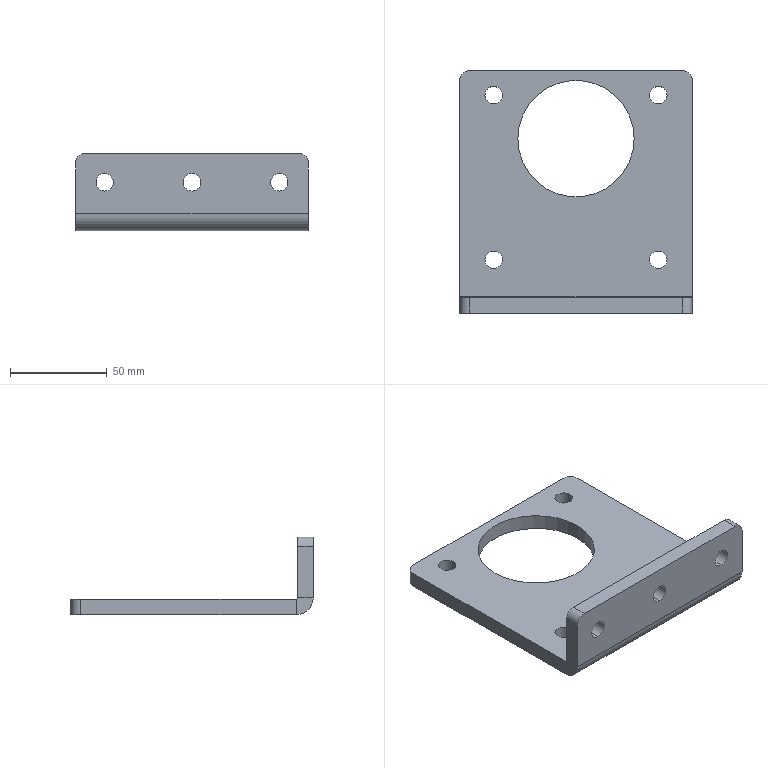Part | SolidWorks | features BaseBody 1 | 1 solid | 34 faces | box 120 x 125 x 40 mm | volume 122415 mm3 | cylinder 22 | plane 12 | commonest cylinder face diameters 9 x14 10 x4 60 x2 1.473 x1 17.473 x1
STEP:
#1=CARTESIAN_POINT('',(0.,-62.5,12.5));
#2=VERTEX_POINT('',#1);
#3=CARTESIAN_POINT('',(0.,-62.5,21.5));
#4=VERTEX_POINT('',#3);
#5=CARTESIAN_POINT('',(0.,-62.5,17.));
#6=DIRECTION('',(0.,1.,0.));
#7=DIRECTION('',(0.,0.,1.));
#8=AXIS2_PLACEMENT_3D('',#5,#6,#7);
#9=CIRCLE('',#8,4.5);
#10=EDGE_CURVE('',#2,#4,#9,.T.);
#11=ORIENTED_EDGE('',*,*,#10,.F.);
#12=CARTESIAN_POINT('',(0.,-54.5,12.5));
#13=VERTEX_POINT('',#12);
#14=CARTESIAN_POINT('',(0.,-54.5,12.5));
#15=DIRECTION('',(0.,1.,0.));
#16=VECTOR('',#15,1000.);
#17=LINE('',#14,#16);
#18=EDGE_CURVE('',#2,#13,#17,.T.);
#19=ORIENTED_EDGE('',*,*,#18,.T.);
#20=CARTESIAN_POINT('',(0.,-54.5,21.5));
#21=VERTEX_POINT('',#20);
#22=CARTESIAN_POINT('',(0.,-54.5,17.));
#23=DIRECTION('',(0.,1.,0.));
#24=DIRECTION('',(0.,0.,1.));
#25=AXIS2_PLACEMENT_3D('',#22,#23,#24);
#26=CIRCLE('',#25,4.5);
#27=EDGE_CURVE('',#13,#21,#26,.T.);
#28=ORIENTED_EDGE('',*,*,#27,.T.);
#29=CARTESIAN_POINT('',(0.,-54.5,21.5));
#30=DIRECTION('',(0.,1.,0.));
#31=VECTOR('',#30,1000.);
#32=LINE('',#29,#31);
#33=EDGE_CURVE('',#4,#21,#32,.T.);
#34=ORIENTED_EDGE('',*,*,#33,.F.);
#35=EDGE_LOOP('',(#11,#19,#28,#34));
#36=FACE_OUTER_BOUND('',#35,.T.);
#37=CARTESIAN_POINT('',(0.,-54.5,17.));
#38=DIRECTION('',(0.,1.,0.));
#39=DIRECTION('',(0.,0.,1.));
#40=AXIS2_PLACEMENT_3D('',#37,#38,#39);
#41=CYLINDRICAL_SURFACE('',#40,4.5);
#42=ADVANCED_FACE('',(#36),#41,.F.);
#43=CARTESIAN_POINT('',(45.,-62.5,12.5));
#44=VERTEX_POINT('',#43);
#45=CARTESIAN_POINT('',(45.,-62.5,21.5));
#46=VERTEX_POINT('',#45);
#47=CARTESIAN_POINT('',(45.,-62.5,17.));
#48=DIRECTION('',(0.,1.,0.));
#49=DIRECTION('',(0.,0.,1.));
#50=AXIS2_PLACEMENT_3D('',#47,#48,#49);
#51=CIRCLE('',#50,4.5);
#52=EDGE_CURVE('',#44,#46,#51,.T.);
#53=ORIENTED_EDGE('',*,*,#52,.F.);
#54=CARTESIAN_POINT('',(45.,-54.5,12.5));
#55=VERTEX_POINT('',#54);
#56=CARTESIAN_POINT('',(45.,-54.5,12.5));
#57=DIRECTION('',(0.,1.,0.));
#58=VECTOR('',#57,1000.);
#59=LINE('',#56,#58);
#60=EDGE_CURVE('',#44,#55,#59,.T.);
#61=ORIENTED_EDGE('',*,*,#60,.T.);
#62=CARTESIAN_POINT('',(45.,-54.5,21.5));
#63=VERTEX_POINT('',#62);
#64=CARTESIAN_POINT('',(45.,-54.5,17.));
#65=DIRECTION('',(0.,1.,0.));
#66=DIRECTION('',(0.,0.,1.));
#67=AXIS2_PLACEMENT_3D('',#64,#65,#66);
#68=CIRCLE('',#67,4.5);
#69=EDGE_CURVE('',#55,#63,#68,.T.);
#70=ORIENTED_EDGE('',*,*,#69,.T.);
#71=CARTESIAN_POINT('',(45.,-54.5,21.5));
#72=DIRECTION('',(0.,1.,0.));
#73=VECTOR('',#72,1000.);
#74=LINE('',#71,#73);
#75=EDGE_CURVE('',#46,#63,#74,.T.);
#76=ORIENTED_EDGE('',*,*,#75,.F.);
#77=EDGE_LOOP('',(#53,#61,#70,#76));
#78=FACE_OUTER_BOUND('',#77,.T.);
#79=CARTESIAN_POINT('',(45.,-54.5,17.));
#80=DIRECTION('',(0.,1.,0.));
#81=DIRECTION('',(0.,0.,1.));
#82=AXIS2_PLACEMENT_3D('',#79,#80,#81);
#83=CYLINDRICAL_SURFACE('',#82,4.5);
#84=ADVANCED_FACE('',(#78),#83,.F.);
#85=CARTESIAN_POINT('',(-45.,-62.5,12.5));
#86=VERTEX_POINT('',#85);
#87=CARTESIAN_POINT('',(-45.,-62.5,21.5));
#88=VERTEX_POINT('',#87);
#89=CARTESIAN_POINT('',(-45.,-62.5,17.));
#90=DIRECTION('',(0.,1.,0.));
#91=DIRECTION('',(0.,0.,1.));
#92=AXIS2_PLACEMENT_3D('',#89,#90,#91);
#93=CIRCLE('',#92,4.5);
#94=EDGE_CURVE('',#86,#88,#93,.T.);
#95=ORIENTED_EDGE('',*,*,#94,.F.);
#96=CARTESIAN_POINT('',(-45.,-54.5,12.5));
#97=VERTEX_POINT('',#96);
#98=CARTESIAN_POINT('',(-45.,-54.5,12.5));
#99=DIRECTION('',(0.,1.,0.));
#100=VECTOR('',#99,1000.);
#101=LINE('',#98,#100);
#102=EDGE_CURVE('',#86,#97,#101,.T.);
#103=ORIENTED_EDGE('',*,*,#102,.T.);
#104=CARTESIAN_POINT('',(-45.,-54.5,21.5));
#105=VERTEX_POINT('',#104);
#106=CARTESIAN_POINT('',(-45.,-54.5,17.));
#107=DIRECTION('',(0.,1.,0.));
#108=DIRECTION('',(0.,0.,1.));
#109=AXIS2_PLACEMENT_3D('',#106,#107,#108);
#110=CIRCLE('',#109,4.5);
#111=EDGE_CURVE('',#97,#105,#110,.T.);
#112=ORIENTED_EDGE('',*,*,#111,.T.);
#113=CARTESIAN_POINT('',(-45.,-54.5,21.5));
#114=DIRECTION('',(0.,1.,0.));
#115=VECTOR('',#114,1000.);
#116=LINE('',#113,#115);
#117=EDGE_CURVE('',#88,#105,#116,.T.);
#118=ORIENTED_EDGE('',*,*,#117,.F.);
#119=EDGE_LOOP('',(#95,#103,#112,#118));
#120=FACE_OUTER_BOUND('',#119,.T.);
#121=CARTESIAN_POINT('',(-45.,-54.5,17.));
#122=DIRECTION('',(0.,1.,0.));
#123=DIRECTION('',(0.,0.,1.));
#124=AXIS2_PLACEMENT_3D('',#121,#122,#123);
#125=CYLINDRICAL_SURFACE('',#124,4.5);
#126=ADVANCED_FACE('',(#120),#125,.F.);
#127=CARTESIAN_POINT('',(-30.,27.5,-8.));
#128=VERTEX_POINT('',#127);
#129=CARTESIAN_POINT('',(30.,27.5,-8.));
#130=VERTEX_POINT('',#129);
#131=CARTESIAN_POINT('',(0.,27.5,-8.));
#132=DIRECTION('',(0.,0.,1.));
#133=DIRECTION('',(1.,0.,0.));
#134=AXIS2_PLACEMENT_3D('',#131,#132,#133);
#135=CIRCLE('',#134,30.);
#136=EDGE_CURVE('',#128,#130,#135,.T.);
#137=ORIENTED_EDGE('',*,*,#136,.F.);
#138=CARTESIAN_POINT('',(-30.,27.5,0.));
#139=VERTEX_POINT('',#138);
#140=CARTESIAN_POINT('',(-30.,27.5,-8.));
#141=DIRECTION('',(0.,0.,1.));
#142=VECTOR('',#141,1000.);
#143=LINE('',#140,#142);
#144=EDGE_CURVE('',#128,#139,#143,.T.);
#145=ORIENTED_EDGE('',*,*,#144,.T.);
#146=CARTESIAN_POINT('',(30.,27.5,0.));
#147=VERTEX_POINT('',#146);
#148=CARTESIAN_POINT('',(0.,27.5,0.));
#149=DIRECTION('',(0.,0.,1.));
#150=DIRECTION('',(1.,0.,0.));
#151=AXIS2_PLACEMENT_3D('',#148,#149,#150);
#152=CIRCLE('',#151,30.);
#153=EDGE_CURVE('',#139,#147,#152,.T.);
#154=ORIENTED_EDGE('',*,*,#153,.T.);
#155=CARTESIAN_POINT('',(30.,27.5,-8.));
#156=DIRECTION('',(0.,0.,1.));
#157=VECTOR('',#156,1000.);
#158=LINE('',#155,#157);
#159=EDGE_CURVE('',#130,#147,#158,.T.);
#160=ORIENTED_EDGE('',*,*,#159,.F.);
#161=EDGE_LOOP('',(#137,#145,#154,#160));
#162=FACE_OUTER_BOUND('',#161,.T.);
#163=CARTESIAN_POINT('',(0.,27.5,-8.));
#164=DIRECTION('',(0.,0.,1.));
#165=DIRECTION('',(1.,0.,0.));
#166=AXIS2_PLACEMENT_3D('',#163,#164,#165);
#167=CYLINDRICAL_SURFACE('',#166,30.);
#168=ADVANCED_FACE('',(#162),#167,.F.);
#169=CARTESIAN_POINT('',(-46.926,-34.926,-8.));
#170=VERTEX_POINT('',#169);
#171=CARTESIAN_POINT('',(-37.926,-34.926,-8.));
#172=VERTEX_POINT('',#171);
#173=CARTESIAN_POINT('',(-42.426,-34.926,-8.));
#174=DIRECTION('',(0.,0.,1.));
#175=DIRECTION('',(1.,0.,0.));
#176=AXIS2_PLACEMENT_3D('',#173,#174,#175);
#177=CIRCLE('',#176,4.5);
#178=EDGE_CURVE('',#170,#172,#177,.T.);
#179=ORIENTED_EDGE('',*,*,#178,.F.);
#180=CARTESIAN_POINT('',(-46.926,-34.926,0.));
#181=VERTEX_POINT('',#180);
#182=CARTESIAN_POINT('',(-46.926,-34.926,-8.));
#183=DIRECTION('',(0.,0.,1.));
#184=VECTOR('',#183,1000.);
#185=LINE('',#182,#184);
#186=EDGE_CURVE('',#170,#181,#185,.T.);
#187=ORIENTED_EDGE('',*,*,#186,.T.);
#188=CARTESIAN_POINT('',(-37.926,-34.926,0.));
#189=VERTEX_POINT('',#188);
#190=CARTESIAN_POINT('',(-42.426,-34.926,0.));
#191=DIRECTION('',(0.,0.,1.));
#192=DIRECTION('',(1.,0.,0.));
#193=AXIS2_PLACEMENT_3D('',#190,#191,#192);
#194=CIRCLE('',#193,4.5);
#195=EDGE_CURVE('',#181,#189,#194,.T.);
#196=ORIENTED_EDGE('',*,*,#195,.T.);
#197=CARTESIAN_POINT('',(-37.926,-34.926,-8.));
#198=DIRECTION('',(0.,0.,1.));
#199=VECTOR('',#198,1000.);
#200=LINE('',#197,#199);
#201=EDGE_CURVE('',#172,#189,#200,.T.);
#202=ORIENTED_EDGE('',*,*,#201,.F.);
#203=EDGE_LOOP('',(#179,#187,#196,#202));
#204=FACE_OUTER_BOUND('',#203,.T.);
#205=CARTESIAN_POINT('',(-42.426,-34.926,-8.));
#206=DIRECTION('',(0.,0.,1.));
#207=DIRECTION('',(1.,0.,0.));
#208=AXIS2_PLACEMENT_3D('',#205,#206,#207);
#209=CYLINDRICAL_SURFACE('',#208,4.5);
#210=ADVANCED_FACE('',(#204),#209,.F.);
#211=CARTESIAN_POINT('',(37.926,-34.926,-8.));
#212=VERTEX_POINT('',#211);
#213=CARTESIAN_POINT('',(46.926,-34.926,-8.));
#214=VERTEX_POINT('',#213);
#215=CARTESIAN_POINT('',(42.426,-34.926,-8.));
#216=DIRECTION('',(0.,0.,1.));
#217=DIRECTION('',(-1.,0.,0.));
#218=AXIS2_PLACEMENT_3D('',#215,#216,#217);
#219=CIRCLE('',#218,4.5);
#220=EDGE_CURVE('',#212,#214,#219,.T.);
#221=ORIENTED_EDGE('',*,*,#220,.F.);
#222=CARTESIAN_POINT('',(37.926,-34.926,0.));
#223=VERTEX_POINT('',#222);
#224=CARTESIAN_POINT('',(37.926,-34.926,-8.));
#225=DIRECTION('',(0.,0.,1.));
#226=VECTOR('',#225,1000.);
#227=LINE('',#224,#226);
#228=EDGE_CURVE('',#212,#223,#227,.T.);
#229=ORIENTED_EDGE('',*,*,#228,.T.);
#230=CARTESIAN_POINT('',(46.926,-34.926,0.));
#231=VERTEX_POINT('',#230);
#232=CARTESIAN_POINT('',(42.426,-34.926,0.));
#233=DIRECTION('',(0.,0.,1.));
#234=DIRECTION('',(-1.,0.,0.));
#235=AXIS2_PLACEMENT_3D('',#232,#233,#234);
#236=CIRCLE('',#235,4.5);
#237=EDGE_CURVE('',#223,#231,#236,.T.);
#238=ORIENTED_EDGE('',*,*,#237,.T.);
#239=CARTESIAN_POINT('',(46.926,-34.926,-8.));
#240=DIRECTION('',(0.,0.,1.));
#241=VECTOR('',#240,1000.);
#242=LINE('',#239,#241);
#243=EDGE_CURVE('',#214,#231,#242,.T.);
#244=ORIENTED_EDGE('',*,*,#243,.F.);
#245=EDGE_LOOP('',(#221,#229,#238,#244));
#246=FACE_OUTER_BOUND('',#245,.T.);
#247=CARTESIAN_POINT('',(42.426,-34.926,-8.));
#248=DIRECTION('',(0.,0.,1.));
#249=DIRECTION('',(1.,0.,0.));
#250=AXIS2_PLACEMENT_3D('',#247,#248,#249);
#251=CYLINDRICAL_SURFACE('',#250,4.5);
#252=ADVANCED_FACE('',(#246),#251,.F.);
#253=CARTESIAN_POINT('',(-46.926,49.926,-8.));
#254=VERTEX_POINT('',#253);
#255=CARTESIAN_POINT('',(-37.926,49.926,-8.));
#256=VERTEX_POINT('',#255);
#257=CARTESIAN_POINT('',(-42.426,49.926,-8.));
#258=DIRECTION('',(0.,0.,1.));
#259=DIRECTION('',(-1.,0.,0.));
#260=AXIS2_PLACEMENT_3D('',#257,#258,#259);
#261=CIRCLE('',#260,4.5);
#262=EDGE_CURVE('',#254,#256,#261,.T.);
#263=ORIENTED_EDGE('',*,*,#262,.F.);
#264=CARTESIAN_POINT('',(-46.926,49.926,0.));
#265=VERTEX_POINT('',#264);
#266=CARTESIAN_POINT('',(-46.926,49.926,-8.));
#267=DIRECTION('',(0.,0.,1.));
#268=VECTOR('',#267,1000.);
#269=LINE('',#266,#268);
#270=EDGE_CURVE('',#254,#265,#269,.T.);
#271=ORIENTED_EDGE('',*,*,#270,.T.);
#272=CARTESIAN_POINT('',(-37.926,49.926,0.));
#273=VERTEX_POINT('',#272);
#274=CARTESIAN_POINT('',(-42.426,49.926,0.));
#275=DIRECTION('',(0.,0.,1.));
#276=DIRECTION('',(-1.,0.,0.));
#277=AXIS2_PLACEMENT_3D('',#274,#275,#276);
#278=CIRCLE('',#277,4.5);
#279=EDGE_CURVE('',#265,#273,#278,.T.);
#280=ORIENTED_EDGE('',*,*,#279,.T.);
#281=CARTESIAN_POINT('',(-37.926,49.926,-8.));
#282=DIRECTION('',(0.,0.,1.));
#283=VECTOR('',#282,1000.);
#284=LINE('',#281,#283);
#285=EDGE_CURVE('',#256,#273,#284,.T.);
#286=ORIENTED_EDGE('',*,*,#285,.F.);
#287=EDGE_LOOP('',(#263,#271,#280,#286));
#288=FACE_OUTER_BOUND('',#287,.T.);
#289=CARTESIAN_POINT('',(-42.426,49.926,-8.));
#290=DIRECTION('',(0.,0.,1.));
#291=DIRECTION('',(1.,0.,0.));
#292=AXIS2_PLACEMENT_3D('',#289,#290,#291);
#293=CYLINDRICAL_SURFACE('',#292,4.5);
#294=ADVANCED_FACE('',(#288),#293,.F.);
#295=CARTESIAN_POINT('',(37.926,49.926,-8.));
#296=VERTEX_POINT('',#295);
#297=CARTESIAN_POINT('',(46.926,49.926,-8.));
#298=VERTEX_POINT('',#297);
#299=CARTESIAN_POINT('',(42.426,49.926,-8.));
#300=DIRECTION('',(0.,0.,1.));
#301=DIRECTION('',(1.,0.,0.));
#302=AXIS2_PLACEMENT_3D('',#299,#300,#301);
#303=CIRCLE('',#302,4.5);
#304=EDGE_CURVE('',#296,#298,#303,.T.);
#305=ORIENTED_EDGE('',*,*,#304,.F.);
#306=CARTESIAN_POINT('',(37.926,49.926,0.));
#307=VERTEX_POINT('',#306);
#308=CARTESIAN_POINT('',(37.926,49.926,-8.));
#309=DIRECTION('',(0.,0.,1.));
#310=VECTOR('',#309,1000.);
#311=LINE('',#308,#310);
#312=EDGE_CURVE('',#296,#307,#311,.T.);
#313=ORIENTED_EDGE('',*,*,#312,.T.);
#314=CARTESIAN_POINT('',(46.926,49.926,0.));
#315=VERTEX_POINT('',#314);
#316=CARTESIAN_POINT('',(42.426,49.926,0.));
#317=DIRECTION('',(0.,0.,1.));
#318=DIRECTION('',(1.,0.,0.));
#319=AXIS2_PLACEMENT_3D('',#316,#317,#318);
#320=CIRCLE('',#319,4.5);
#321=EDGE_CURVE('',#307,#315,#320,.T.);
#322=ORIENTED_EDGE('',*,*,#321,.T.);
#323=CARTESIAN_POINT('',(46.926,49.926,-8.));
#324=DIRECTION('',(0.,0.,1.));
#325=VECTOR('',#324,1000.);
#326=LINE('',#323,#325);
#327=EDGE_CURVE('',#298,#315,#326,.T.);
#328=ORIENTED_EDGE('',*,*,#327,.F.);
#329=EDGE_LOOP('',(#305,#313,#322,#328));
#330=FACE_OUTER_BOUND('',#329,.T.);
#331=CARTESIAN_POINT('',(42.426,49.926,-8.));
#332=DIRECTION('',(0.,0.,1.));
#333=DIRECTION('',(1.,0.,0.));
#334=AXIS2_PLACEMENT_3D('',#331,#332,#333);
#335=CYLINDRICAL_SURFACE('',#334,4.5);
#336=ADVANCED_FACE('',(#330),#335,.F.);
#337=CARTESIAN_POINT('',(60.,-53.763,-8.));
#338=VERTEX_POINT('',#337);
#339=CARTESIAN_POINT('',(60.,57.5,-8.));
#340=VERTEX_POINT('',#339);
#341=CARTESIAN_POINT('',(60.,62.5,-8.));
#342=DIRECTION('',(0.,1.,0.));
#343=VECTOR('',#342,1000.);
#344=LINE('',#341,#343);
#345=EDGE_CURVE('',#338,#340,#344,.T.);
#346=ORIENTED_EDGE('',*,*,#345,.T.);
#347=CARTESIAN_POINT('',(60.,57.5,0.));
#348=VERTEX_POINT('',#347);
#349=CARTESIAN_POINT('',(60.,57.5,-8.));
#350=DIRECTION('',(0.,0.,1.));
#351=VECTOR('',#350,1000.);
#352=LINE('',#349,#351);
#353=EDGE_CURVE('',#340,#348,#352,.T.);
#354=ORIENTED_EDGE('',*,*,#353,.T.);
#355=CARTESIAN_POINT('',(60.,-53.763,0.));
#356=VERTEX_POINT('',#355);
#357=CARTESIAN_POINT('',(60.,62.5,0.));
#358=DIRECTION('',(0.,1.,0.));
#359=VECTOR('',#358,1000.);
#360=LINE('',#357,#359);
#361=EDGE_CURVE('',#356,#348,#360,.T.);
#362=ORIENTED_EDGE('',*,*,#361,.F.);
#363=CARTESIAN_POINT('',(60.,-53.763,0.));
#364=DIRECTION('',(0.,0.,-1.));
#365=VECTOR('',#364,1000.);
#366=LINE('',#363,#365);
#367=EDGE_CURVE('',#356,#338,#366,.T.);
#368=ORIENTED_EDGE('',*,*,#367,.T.);
#369=EDGE_LOOP('',(#346,#354,#362,#368));
#370=FACE_OUTER_BOUND('',#369,.T.);
#371=CARTESIAN_POINT('',(60.,62.5,-8.));
#372=DIRECTION('',(1.,0.,0.));
#373=DIRECTION('',(0.,1.,0.));
#374=AXIS2_PLACEMENT_3D('',#371,#372,#373);
#375=PLANE('',#374);
#376=ADVANCED_FACE('',(#370),#375,.T.);
#377=CARTESIAN_POINT('',(42.426,49.926,-8.));
#378=DIRECTION('',(0.,0.,1.));
#379=DIRECTION('',(1.,0.,0.));
#380=AXIS2_PLACEMENT_3D('',#377,#378,#379);
#381=CIRCLE('',#380,4.5);
#382=EDGE_CURVE('',#298,#296,#381,.T.);
#383=ORIENTED_EDGE('',*,*,#382,.T.);
#384=ORIENTED_EDGE('',*,*,#304,.T.);
#385=EDGE_LOOP('',(#383,#384));
#386=FACE_BOUND('',#385,.T.);
#387=CARTESIAN_POINT('',(-42.426,49.926,-8.));
#388=DIRECTION('',(0.,0.,1.));
#389=DIRECTION('',(-1.,0.,0.));
#390=AXIS2_PLACEMENT_3D('',#387,#388,#389);
#391=CIRCLE('',#390,4.5);
#392=EDGE_CURVE('',#256,#254,#391,.T.);
#393=ORIENTED_EDGE('',*,*,#392,.T.);
#394=ORIENTED_EDGE('',*,*,#262,.T.);
#395=EDGE_LOOP('',(#393,#394));
#396=FACE_BOUND('',#395,.T.);
#397=CARTESIAN_POINT('',(42.426,-34.926,-8.));
#398=DIRECTION('',(0.,0.,1.));
#399=DIRECTION('',(-1.,0.,0.));
#400=AXIS2_PLACEMENT_3D('',#397,#398,#399);
#401=CIRCLE('',#400,4.5);
#402=EDGE_CURVE('',#214,#212,#401,.T.);
#403=ORIENTED_EDGE('',*,*,#402,.T.);
#404=ORIENTED_EDGE('',*,*,#220,.T.);
#405=EDGE_LOOP('',(#403,#404));
#406=FACE_BOUND('',#405,.T.);
#407=CARTESIAN_POINT('',(-42.426,-34.926,-8.));
#408=DIRECTION('',(0.,0.,1.));
#409=DIRECTION('',(1.,0.,0.));
#410=AXIS2_PLACEMENT_3D('',#407,#408,#409);
#411=CIRCLE('',#410,4.5);
#412=EDGE_CURVE('',#172,#170,#411,.T.);
#413=ORIENTED_EDGE('',*,*,#412,.T.);
#414=ORIENTED_EDGE('',*,*,#178,.T.);
#415=EDGE_LOOP('',(#413,#414));
#416=FACE_BOUND('',#415,.T.);
#417=CARTESIAN_POINT('',(0.,27.5,-8.));
#418=DIRECTION('',(0.,0.,1.));
#419=DIRECTION('',(1.,0.,0.));
#420=AXIS2_PLACEMENT_3D('',#417,#418,#419);
#421=CIRCLE('',#420,30.);
#422=EDGE_CURVE('',#130,#128,#421,.T.);
#423=ORIENTED_EDGE('',*,*,#422,.T.);
#424=ORIENTED_EDGE('',*,*,#136,.T.);
#425=EDGE_LOOP('',(#423,#424));
#426=FACE_BOUND('',#425,.T.);
#427=CARTESIAN_POINT('',(-60.,57.5,-8.));
#428=VERTEX_POINT('',#427);
#429=CARTESIAN_POINT('',(-60.,-53.763,-8.));
#430=VERTEX_POINT('',#429);
#431=CARTESIAN_POINT('',(-60.,62.5,-8.));
#432=DIRECTION('',(0.,-1.,0.));
#433=VECTOR('',#432,1000.);
#434=LINE('',#431,#433);
#435=EDGE_CURVE('',#428,#430,#434,.T.);
#436=ORIENTED_EDGE('',*,*,#435,.F.);
#437=CARTESIAN_POINT('',(-55.,62.5,-8.));
#438=VERTEX_POINT('',#437);
#439=CARTESIAN_POINT('',(-55.,57.5,-8.));
#440=DIRECTION('',(0.,0.,-1.));
#441=DIRECTION('',(1.,0.,0.));
#442=AXIS2_PLACEMENT_3D('',#439,#440,#441);
#443=CIRCLE('',#442,5.);
#444=EDGE_CURVE('',#428,#438,#443,.T.);
#445=ORIENTED_EDGE('',*,*,#444,.T.);
#446=CARTESIAN_POINT('',(55.,62.5,-8.));
#447=VERTEX_POINT('',#446);
#448=CARTESIAN_POINT('',(-60.,62.5,-8.));
#449=DIRECTION('',(-1.,0.,0.));
#450=VECTOR('',#449,1000.);
#451=LINE('',#448,#450);
#452=EDGE_CURVE('',#447,#438,#451,.T.);
#453=ORIENTED_EDGE('',*,*,#452,.F.);
#454=CARTESIAN_POINT('',(55.,57.5,-8.));
#455=DIRECTION('',(0.,0.,-1.));
#456=DIRECTION('',(1.,0.,0.));
#457=AXIS2_PLACEMENT_3D('',#454,#455,#456);
#458=CIRCLE('',#457,5.);
#459=EDGE_CURVE('',#447,#340,#458,.T.);
#460=ORIENTED_EDGE('',*,*,#459,.T.);
#461=ORIENTED_EDGE('',*,*,#345,.F.);
#462=CARTESIAN_POINT('',(60.,-53.763,-8.));
#463=DIRECTION('',(-1.,0.,0.));
#464=VECTOR('',#463,1000.);
#465=LINE('',#462,#464);
#466=EDGE_CURVE('',#338,#430,#465,.T.);
#467=ORIENTED_EDGE('',*,*,#466,.T.);
#468=EDGE_LOOP('',(#436,#445,#453,#460,#461,#467));
#469=FACE_OUTER_BOUND('',#468,.T.);
#470=CARTESIAN_POINT('',(0.,0.,-8.));
#471=DIRECTION('',(0.,0.,1.));
#472=DIRECTION('',(1.,0.,0.));
#473=AXIS2_PLACEMENT_3D('',#470,#471,#472);
#474=PLANE('',#473);
#475=ADVANCED_FACE('',(#386,#396,#406,#416,#426,#469),#474,.F.);
#476=CARTESIAN_POINT('',(0.,27.5,0.));
#477=DIRECTION('',(0.,0.,1.));
#478=DIRECTION('',(1.,0.,0.));
#479=AXIS2_PLACEMENT_3D('',#476,#477,#478);
#480=CIRCLE('',#479,30.);
#481=EDGE_CURVE('',#147,#139,#480,.T.);
#482=ORIENTED_EDGE('',*,*,#481,.F.);
#483=ORIENTED_EDGE('',*,*,#153,.F.);
#484=EDGE_LOOP('',(#482,#483));
#485=FACE_BOUND('',#484,.T.);
#486=CARTESIAN_POINT('',(-42.426,-34.926,0.));
#487=DIRECTION('',(0.,0.,1.));
#488=DIRECTION('',(1.,0.,0.));
#489=AXIS2_PLACEMENT_3D('',#486,#487,#488);
#490=CIRCLE('',#489,4.5);
#491=EDGE_CURVE('',#189,#181,#490,.T.);
#492=ORIENTED_EDGE('',*,*,#491,.F.);
#493=ORIENTED_EDGE('',*,*,#195,.F.);
#494=EDGE_LOOP('',(#492,#493));
#495=FACE_BOUND('',#494,.T.);
#496=CARTESIAN_POINT('',(42.426,-34.926,0.));
#497=DIRECTION('',(0.,0.,1.));
#498=DIRECTION('',(-1.,0.,0.));
#499=AXIS2_PLACEMENT_3D('',#496,#497,#498);
#500=CIRCLE('',#499,4.5);
#501=EDGE_CURVE('',#231,#223,#500,.T.);
#502=ORIENTED_EDGE('',*,*,#501,.F.);
#503=ORIENTED_EDGE('',*,*,#237,.F.);
#504=EDGE_LOOP('',(#502,#503));
#505=FACE_BOUND('',#504,.T.);
#506=CARTESIAN_POINT('',(-42.426,49.926,0.));
#507=DIRECTION('',(0.,0.,1.));
#508=DIRECTION('',(-1.,0.,0.));
#509=AXIS2_PLACEMENT_3D('',#506,#507,#508);
#510=CIRCLE('',#509,4.5);
#511=EDGE_CURVE('',#273,#265,#510,.T.);
#512=ORIENTED_EDGE('',*,*,#511,.F.);
#513=ORIENTED_EDGE('',*,*,#279,.F.);
#514=EDGE_LOOP('',(#512,#513));
#515=FACE_BOUND('',#514,.T.);
#516=CARTESIAN_POINT('',(42.426,49.926,0.));
#517=DIRECTION('',(0.,0.,1.));
#518=DIRECTION('',(1.,0.,0.));
#519=AXIS2_PLACEMENT_3D('',#516,#517,#518);
#520=CIRCLE('',#519,4.5);
#521=EDGE_CURVE('',#315,#307,#520,.T.);
#522=ORIENTED_EDGE('',*,*,#521,.F.);
#523=ORIENTED_EDGE('',*,*,#321,.F.);
#524=EDGE_LOOP('',(#522,#523));
#525=FACE_BOUND('',#524,.T.);
#526=CARTESIAN_POINT('',(55.,62.5,0.));
#527=VERTEX_POINT('',#526);
#528=CARTESIAN_POINT('',(-55.,62.5,0.));
#529=VERTEX_POINT('',#528);
#530=CARTESIAN_POINT('',(-60.,62.5,0.));
#531=DIRECTION('',(-1.,0.,0.));
#532=VECTOR('',#531,1000.);
#533=LINE('',#530,#532);
#534=EDGE_CURVE('',#527,#529,#533,.T.);
#535=ORIENTED_EDGE('',*,*,#534,.T.);
#536=CARTESIAN_POINT('',(-60.,57.5,0.));
#537=VERTEX_POINT('',#536);
#538=CARTESIAN_POINT('',(-55.,57.5,0.));
#539=DIRECTION('',(0.,0.,1.));
#540=DIRECTION('',(1.,0.,0.));
#541=AXIS2_PLACEMENT_3D('',#538,#539,#540);
#542=CIRCLE('',#541,5.);
#543=EDGE_CURVE('',#529,#537,#542,.T.);
#544=ORIENTED_EDGE('',*,*,#543,.T.);
#545=CARTESIAN_POINT('',(-60.,-53.763,0.));
#546=VERTEX_POINT('',#545);
#547=CARTESIAN_POINT('',(-60.,62.5,0.));
#548=DIRECTION('',(0.,-1.,0.));
#549=VECTOR('',#548,1000.);
#550=LINE('',#547,#549);
#551=EDGE_CURVE('',#537,#546,#550,.T.);
#552=ORIENTED_EDGE('',*,*,#551,.T.);
#553=CARTESIAN_POINT('',(60.,-53.763,0.));
#554=DIRECTION('',(-1.,0.,0.));
#555=VECTOR('',#554,1000.);
#556=LINE('',#553,#555);
#557=EDGE_CURVE('',#356,#546,#556,.T.);
#558=ORIENTED_EDGE('',*,*,#557,.F.);
#559=ORIENTED_EDGE('',*,*,#361,.T.);
#560=CARTESIAN_POINT('',(55.,57.5,0.));
#561=DIRECTION('',(0.,0.,1.));
#562=DIRECTION('',(1.,0.,0.));
#563=AXIS2_PLACEMENT_3D('',#560,#561,#562);
#564=CIRCLE('',#563,5.);
#565=EDGE_CURVE('',#348,#527,#564,.T.);
#566=ORIENTED_EDGE('',*,*,#565,.T.);
#567=EDGE_LOOP('',(#535,#544,#552,#558,#559,#566));
#568=FACE_OUTER_BOUND('',#567,.T.);
#569=CARTESIAN_POINT('',(0.,0.,0.));
#570=DIRECTION('',(0.,0.,1.));
#571=DIRECTION('',(1.,0.,0.));
#572=AXIS2_PLACEMENT_3D('',#569,#570,#571);
#573=PLANE('',#572);
#574=ADVANCED_FACE('',(#485,#495,#505,#515,#525,#568),#573,.T.);
#575=ORIENTED_EDGE('',*,*,#551,.F.);
#576=CARTESIAN_POINT('',(-60.,57.5,-8.));
#577=DIRECTION('',(0.,0.,-1.));
#578=VECTOR('',#577,1000.);
#579=LINE('',#576,#578);
#580=EDGE_CURVE('',#537,#428,#579,.T.);
#581=ORIENTED_EDGE('',*,*,#580,.T.);
#582=ORIENTED_EDGE('',*,*,#435,.T.);
#583=CARTESIAN_POINT('',(-60.,-53.763,0.));
#584=DIRECTION('',(0.,0.,-1.));
#585=VECTOR('',#584,1000.);
#586=LINE('',#583,#585);
#587=EDGE_CURVE('',#546,#430,#586,.T.);
#588=ORIENTED_EDGE('',*,*,#587,.F.);
#589=EDGE_LOOP('',(#575,#581,#582,#588));
#590=FACE_OUTER_BOUND('',#589,.T.);
#591=CARTESIAN_POINT('',(-60.,62.5,-8.));
#592=DIRECTION('',(-1.,0.,0.));
#593=DIRECTION('',(0.,-1.,0.));
#594=AXIS2_PLACEMENT_3D('',#591,#592,#593);
#595=PLANE('',#594);
#596=ADVANCED_FACE('',(#590),#595,.T.);
#597=ORIENTED_EDGE('',*,*,#452,.T.);
#598=CARTESIAN_POINT('',(-55.,62.5,-8.));
#599=DIRECTION('',(0.,0.,1.));
#600=VECTOR('',#599,1000.);
#601=LINE('',#598,#600);
#602=EDGE_CURVE('',#438,#529,#601,.T.);
#603=ORIENTED_EDGE('',*,*,#602,.T.);
#604=ORIENTED_EDGE('',*,*,#534,.F.);
#605=CARTESIAN_POINT('',(55.,62.5,-8.));
#606=DIRECTION('',(0.,0.,-1.));
#607=VECTOR('',#606,1000.);
#608=LINE('',#605,#607);
#609=EDGE_CURVE('',#527,#447,#608,.T.);
#610=ORIENTED_EDGE('',*,*,#609,.T.);
#611=EDGE_LOOP('',(#597,#603,#604,#610));
#612=FACE_OUTER_BOUND('',#611,.T.);
#613=CARTESIAN_POINT('',(-60.,62.5,-8.));
#614=DIRECTION('',(0.,1.,0.));
#615=DIRECTION('',(0.,0.,1.));
#616=AXIS2_PLACEMENT_3D('',#613,#614,#615);
#617=PLANE('',#616);
#618=ADVANCED_FACE('',(#612),#617,.T.);
#619=ORIENTED_EDGE('',*,*,#312,.F.);
#620=ORIENTED_EDGE('',*,*,#382,.F.);
#621=ORIENTED_EDGE('',*,*,#327,.T.);
#622=ORIENTED_EDGE('',*,*,#521,.T.);
#623=EDGE_LOOP('',(#619,#620,#621,#622));
#624=FACE_OUTER_BOUND('',#623,.T.);
#625=CARTESIAN_POINT('',(42.426,49.926,-8.));
#626=DIRECTION('',(0.,0.,1.));
#627=DIRECTION('',(1.,0.,0.));
#628=AXIS2_PLACEMENT_3D('',#625,#626,#627);
#629=CYLINDRICAL_SURFACE('',#628,4.5);
#630=ADVANCED_FACE('',(#624),#629,.F.);
#631=ORIENTED_EDGE('',*,*,#270,.F.);
#632=ORIENTED_EDGE('',*,*,#392,.F.);
#633=ORIENTED_EDGE('',*,*,#285,.T.);
#634=ORIENTED_EDGE('',*,*,#511,.T.);
#635=EDGE_LOOP('',(#631,#632,#633,#634));
#636=FACE_OUTER_BOUND('',#635,.T.);
#637=CARTESIAN_POINT('',(-42.426,49.926,-8.));
#638=DIRECTION('',(0.,0.,1.));
#639=DIRECTION('',(1.,0.,0.));
#640=AXIS2_PLACEMENT_3D('',#637,#638,#639);
#641=CYLINDRICAL_SURFACE('',#640,4.5);
#642=ADVANCED_FACE('',(#636),#641,.F.);
#643=ORIENTED_EDGE('',*,*,#228,.F.);
#644=ORIENTED_EDGE('',*,*,#402,.F.);
#645=ORIENTED_EDGE('',*,*,#243,.T.);
#646=ORIENTED_EDGE('',*,*,#501,.T.);
#647=EDGE_LOOP('',(#643,#644,#645,#646));
#648=FACE_OUTER_BOUND('',#647,.T.);
#649=CARTESIAN_POINT('',(42.426,-34.926,-8.));
#650=DIRECTION('',(0.,0.,1.));
#651=DIRECTION('',(1.,0.,0.));
#652=AXIS2_PLACEMENT_3D('',#649,#650,#651);
#653=CYLINDRICAL_SURFACE('',#652,4.5);
#654=ADVANCED_FACE('',(#648),#653,.F.);
#655=ORIENTED_EDGE('',*,*,#186,.F.);
#656=ORIENTED_EDGE('',*,*,#412,.F.);
#657=ORIENTED_EDGE('',*,*,#201,.T.);
#658=ORIENTED_EDGE('',*,*,#491,.T.);
#659=EDGE_LOOP('',(#655,#656,#657,#658));
#660=FACE_OUTER_BOUND('',#659,.T.);
#661=CARTESIAN_POINT('',(-42.426,-34.926,-8.));
#662=DIRECTION('',(0.,0.,1.));
#663=DIRECTION('',(1.,0.,0.));
#664=AXIS2_PLACEMENT_3D('',#661,#662,#663);
#665=CYLINDRICAL_SURFACE('',#664,4.5);
#666=ADVANCED_FACE('',(#660),#665,.F.);
#667=ORIENTED_EDGE('',*,*,#144,.F.);
#668=ORIENTED_EDGE('',*,*,#422,.F.);
#669=ORIENTED_EDGE('',*,*,#159,.T.);
#670=ORIENTED_EDGE('',*,*,#481,.T.);
#671=EDGE_LOOP('',(#667,#668,#669,#670));
#672=FACE_OUTER_BOUND('',#671,.T.);
#673=CARTESIAN_POINT('',(0.,27.5,-8.));
#674=DIRECTION('',(0.,0.,1.));
#675=DIRECTION('',(1.,0.,0.));
#676=AXIS2_PLACEMENT_3D('',#673,#674,#675);
#677=CYLINDRICAL_SURFACE('',#676,30.);
#678=ADVANCED_FACE('',(#672),#677,.F.);
#679=CARTESIAN_POINT('',(-60.,-54.5,0.7366));
#680=VERTEX_POINT('',#679);
#681=CARTESIAN_POINT('',(-60.,-62.5,0.7366));
#682=VERTEX_POINT('',#681);
#683=CARTESIAN_POINT('',(-60.,-62.5,0.7366));
#684=DIRECTION('',(0.,-1.,0.));
#685=VECTOR('',#684,1000.);
#686=LINE('',#683,#685);
#687=EDGE_CURVE('',#680,#682,#686,.T.);
#688=ORIENTED_EDGE('',*,*,#687,.F.);
#689=CARTESIAN_POINT('',(-60.,-53.763,0.7366));
#690=DIRECTION('',(-1.,0.,0.));
#691=DIRECTION('',(0.,0.,-1.));
#692=AXIS2_PLACEMENT_3D('',#689,#690,#691);
#693=CIRCLE('',#692,0.7366);
#694=EDGE_CURVE('',#546,#680,#693,.T.);
#695=ORIENTED_EDGE('',*,*,#694,.F.);
#696=ORIENTED_EDGE('',*,*,#587,.T.);
#697=CARTESIAN_POINT('',(-60.,-53.763,0.7366));
#698=DIRECTION('',(-1.,0.,0.));
#699=DIRECTION('',(0.,0.,-1.));
#700=AXIS2_PLACEMENT_3D('',#697,#698,#699);
#701=CIRCLE('',#700,8.737);
#702=EDGE_CURVE('',#430,#682,#701,.T.);
#703=ORIENTED_EDGE('',*,*,#702,.T.);
#704=EDGE_LOOP('',(#688,#695,#696,#703));
#705=FACE_OUTER_BOUND('',#704,.T.);
#706=CARTESIAN_POINT('',(-60.,-53.763,0.7366));
#707=DIRECTION('',(-1.,0.,0.));
#708=DIRECTION('',(0.,0.,1.));
#709=AXIS2_PLACEMENT_3D('',#706,#707,#708);
#710=PLANE('',#709);
#711=ADVANCED_FACE('',(#705),#710,.T.);
#712=CARTESIAN_POINT('',(60.,-54.5,0.7366));
#713=VERTEX_POINT('',#712);
#714=CARTESIAN_POINT('',(60.,-53.763,0.7366));
#715=DIRECTION('',(1.,0.,0.));
#716=DIRECTION('',(0.,0.,-1.));
#717=AXIS2_PLACEMENT_3D('',#714,#715,#716);
#718=CIRCLE('',#717,0.7366);
#719=EDGE_CURVE('',#713,#356,#718,.T.);
#720=ORIENTED_EDGE('',*,*,#719,.F.);
#721=CARTESIAN_POINT('',(60.,-62.5,0.7366));
#722=VERTEX_POINT('',#721);
#723=CARTESIAN_POINT('',(60.,-54.5,0.7366));
#724=DIRECTION('',(0.,-1.,0.));
#725=VECTOR('',#724,1000.);
#726=LINE('',#723,#725);
#727=EDGE_CURVE('',#713,#722,#726,.T.);
#728=ORIENTED_EDGE('',*,*,#727,.T.);
#729=CARTESIAN_POINT('',(60.,-53.763,0.7366));
#730=DIRECTION('',(1.,0.,0.));
#731=DIRECTION('',(0.,0.,-1.));
#732=AXIS2_PLACEMENT_3D('',#729,#730,#731);
#733=CIRCLE('',#732,8.737);
#734=EDGE_CURVE('',#722,#338,#733,.T.);
#735=ORIENTED_EDGE('',*,*,#734,.T.);
#736=ORIENTED_EDGE('',*,*,#367,.F.);
#737=EDGE_LOOP('',(#720,#728,#735,#736));
#738=FACE_OUTER_BOUND('',#737,.T.);
#739=CARTESIAN_POINT('',(60.,-53.763,0.7366));
#740=DIRECTION('',(-1.,0.,0.));
#741=DIRECTION('',(0.,0.,1.));
#742=AXIS2_PLACEMENT_3D('',#739,#740,#741);
#743=PLANE('',#742);
#744=ADVANCED_FACE('',(#738),#743,.F.);
#745=ORIENTED_EDGE('',*,*,#466,.F.);
#746=ORIENTED_EDGE('',*,*,#734,.F.);
#747=CARTESIAN_POINT('',(-60.,-62.5,0.7366));
#748=DIRECTION('',(-1.,0.,0.));
#749=VECTOR('',#748,1000.);
#750=LINE('',#747,#749);
#751=EDGE_CURVE('',#722,#682,#750,.T.);
#752=ORIENTED_EDGE('',*,*,#751,.T.);
#753=ORIENTED_EDGE('',*,*,#702,.F.);
#754=EDGE_LOOP('',(#745,#746,#752,#753));
#755=FACE_OUTER_BOUND('',#754,.T.);
#756=CARTESIAN_POINT('',(60.,-53.763,0.7366));
#757=DIRECTION('',(1.,0.,0.));
#758=DIRECTION('',(0.,-1.,0.));
#759=AXIS2_PLACEMENT_3D('',#756,#757,#758);
#760=CYLINDRICAL_SURFACE('',#759,8.737);
#761=ADVANCED_FACE('',(#755),#760,.T.);
#762=ORIENTED_EDGE('',*,*,#557,.T.);
#763=ORIENTED_EDGE('',*,*,#694,.T.);
#764=CARTESIAN_POINT('',(-60.,-54.5,0.7366));
#765=DIRECTION('',(1.,0.,0.));
#766=VECTOR('',#765,1000.);
#767=LINE('',#764,#766);
#768=EDGE_CURVE('',#680,#713,#767,.T.);
#769=ORIENTED_EDGE('',*,*,#768,.T.);
#770=ORIENTED_EDGE('',*,*,#719,.T.);
#771=EDGE_LOOP('',(#762,#763,#769,#770));
#772=FACE_OUTER_BOUND('',#771,.T.);
#773=CARTESIAN_POINT('',(60.,-53.763,0.7366));
#774=DIRECTION('',(1.,0.,0.));
#775=DIRECTION('',(0.,-1.,0.));
#776=AXIS2_PLACEMENT_3D('',#773,#774,#775);
#777=CYLINDRICAL_SURFACE('',#776,0.7366);
#778=ADVANCED_FACE('',(#772),#777,.F.);
#779=CARTESIAN_POINT('',(-60.,-62.5,27.));
#780=VERTEX_POINT('',#779);
#781=CARTESIAN_POINT('',(-60.,-62.5,0.));
#782=DIRECTION('',(0.,0.,-1.));
#783=VECTOR('',#782,1000.);
#784=LINE('',#781,#783);
#785=EDGE_CURVE('',#780,#682,#784,.T.);
#786=ORIENTED_EDGE('',*,*,#785,.F.);
#787=CARTESIAN_POINT('',(-60.,-54.5,27.));
#788=VERTEX_POINT('',#787);
#789=CARTESIAN_POINT('',(-60.,-62.5,27.));
#790=DIRECTION('',(0.,1.,0.));
#791=VECTOR('',#790,1000.);
#792=LINE('',#789,#791);
#793=EDGE_CURVE('',#780,#788,#792,.T.);
#794=ORIENTED_EDGE('',*,*,#793,.T.);
#795=CARTESIAN_POINT('',(-60.,-54.5,0.));
#796=DIRECTION('',(0.,0.,-1.));
#797=VECTOR('',#796,1000.);
#798=LINE('',#795,#797);
#799=EDGE_CURVE('',#788,#680,#798,.T.);
#800=ORIENTED_EDGE('',*,*,#799,.T.);
#801=ORIENTED_EDGE('',*,*,#687,.T.);
#802=EDGE_LOOP('',(#786,#794,#800,#801));
#803=FACE_OUTER_BOUND('',#802,.T.);
#804=CARTESIAN_POINT('',(-60.,-62.5,0.));
#805=DIRECTION('',(1.,0.,0.));
#806=DIRECTION('',(0.,0.,-1.));
#807=AXIS2_PLACEMENT_3D('',#804,#805,#806);
#808=PLANE('',#807);
#809=ADVANCED_FACE('',(#803),#808,.F.);
#810=CARTESIAN_POINT('',(60.,-54.5,27.));
#811=VERTEX_POINT('',#810);
#812=CARTESIAN_POINT('',(60.,-54.5,32.));
#813=DIRECTION('',(0.,0.,1.));
#814=VECTOR('',#813,1000.);
#815=LINE('',#812,#814);
#816=EDGE_CURVE('',#713,#811,#815,.T.);
#817=ORIENTED_EDGE('',*,*,#816,.T.);
#818=CARTESIAN_POINT('',(60.,-62.5,27.));
#819=VERTEX_POINT('',#818);
#820=CARTESIAN_POINT('',(60.,-62.5,27.));
#821=DIRECTION('',(0.,-1.,0.));
#822=VECTOR('',#821,1000.);
#823=LINE('',#820,#822);
#824=EDGE_CURVE('',#811,#819,#823,.T.);
#825=ORIENTED_EDGE('',*,*,#824,.T.);
#826=CARTESIAN_POINT('',(60.,-62.5,0.));
#827=DIRECTION('',(0.,0.,1.));
#828=VECTOR('',#827,1000.);
#829=LINE('',#826,#828);
#830=EDGE_CURVE('',#722,#819,#829,.T.);
#831=ORIENTED_EDGE('',*,*,#830,.F.);
#832=ORIENTED_EDGE('',*,*,#727,.F.);
#833=EDGE_LOOP('',(#817,#825,#831,#832));
#834=FACE_OUTER_BOUND('',#833,.T.);
#835=CARTESIAN_POINT('',(60.,-62.5,32.));
#836=DIRECTION('',(-1.,0.,0.));
#837=DIRECTION('',(0.,-1.,0.));
#838=AXIS2_PLACEMENT_3D('',#835,#836,#837);
#839=PLANE('',#838);
#840=ADVANCED_FACE('',(#834),#839,.F.);
#841=CARTESIAN_POINT('',(0.,-62.5,17.));
#842=DIRECTION('',(0.,1.,0.));
#843=DIRECTION('',(0.,0.,1.));
#844=AXIS2_PLACEMENT_3D('',#841,#842,#843);
#845=CIRCLE('',#844,4.5);
#846=EDGE_CURVE('',#4,#2,#845,.T.);
#847=ORIENTED_EDGE('',*,*,#846,.T.);
#848=ORIENTED_EDGE('',*,*,#10,.T.);
#849=EDGE_LOOP('',(#847,#848));
#850=FACE_BOUND('',#849,.T.);
#851=CARTESIAN_POINT('',(45.,-62.5,17.));
#852=DIRECTION('',(0.,1.,0.));
#853=DIRECTION('',(0.,0.,1.));
#854=AXIS2_PLACEMENT_3D('',#851,#852,#853);
#855=CIRCLE('',#854,4.5);
#856=EDGE_CURVE('',#46,#44,#855,.T.);
#857=ORIENTED_EDGE('',*,*,#856,.T.);
#858=ORIENTED_EDGE('',*,*,#52,.T.);
#859=EDGE_LOOP('',(#857,#858));
#860=FACE_BOUND('',#859,.T.);
#861=CARTESIAN_POINT('',(-45.,-62.5,17.));
#862=DIRECTION('',(0.,1.,0.));
#863=DIRECTION('',(0.,0.,1.));
#864=AXIS2_PLACEMENT_3D('',#861,#862,#863);
#865=CIRCLE('',#864,4.5);
#866=EDGE_CURVE('',#88,#86,#865,.T.);
#867=ORIENTED_EDGE('',*,*,#866,.T.);
#868=ORIENTED_EDGE('',*,*,#94,.T.);
#869=EDGE_LOOP('',(#867,#868));
#870=FACE_BOUND('',#869,.T.);
#871=ORIENTED_EDGE('',*,*,#830,.T.);
#872=CARTESIAN_POINT('',(55.,-62.5,32.));
#873=VERTEX_POINT('',#872);
#874=CARTESIAN_POINT('',(55.,-62.5,27.));
#875=DIRECTION('',(0.,-1.,0.));
#876=DIRECTION('',(0.,0.,1.));
#877=AXIS2_PLACEMENT_3D('',#874,#875,#876);
#878=CIRCLE('',#877,5.);
#879=EDGE_CURVE('',#819,#873,#878,.T.);
#880=ORIENTED_EDGE('',*,*,#879,.T.);
#881=CARTESIAN_POINT('',(-55.,-62.5,32.));
#882=VERTEX_POINT('',#881);
#883=CARTESIAN_POINT('',(0.,-62.5,32.));
#884=DIRECTION('',(-1.,0.,0.));
#885=VECTOR('',#884,1000.);
#886=LINE('',#883,#885);
#887=EDGE_CURVE('',#873,#882,#886,.T.);
#888=ORIENTED_EDGE('',*,*,#887,.T.);
#889=CARTESIAN_POINT('',(-55.,-62.5,27.));
#890=DIRECTION('',(0.,-1.,0.));
#891=DIRECTION('',(0.,0.,1.));
#892=AXIS2_PLACEMENT_3D('',#889,#890,#891);
#893=CIRCLE('',#892,5.);
#894=EDGE_CURVE('',#882,#780,#893,.T.);
#895=ORIENTED_EDGE('',*,*,#894,.T.);
#896=ORIENTED_EDGE('',*,*,#785,.T.);
#897=ORIENTED_EDGE('',*,*,#751,.F.);
#898=EDGE_LOOP('',(#871,#880,#888,#895,#896,#897));
#899=FACE_OUTER_BOUND('',#898,.T.);
#900=CARTESIAN_POINT('',(0.,-62.5,0.));
#901=DIRECTION('',(0.,1.,0.));
#902=DIRECTION('',(0.,0.,1.));
#903=AXIS2_PLACEMENT_3D('',#900,#901,#902);
#904=PLANE('',#903);
#905=ADVANCED_FACE('',(#850,#860,#870,#899),#904,.F.);
#906=CARTESIAN_POINT('',(0.,-54.5,17.));
#907=DIRECTION('',(0.,1.,0.));
#908=DIRECTION('',(0.,0.,1.));
#909=AXIS2_PLACEMENT_3D('',#906,#907,#908);
#910=CIRCLE('',#909,4.5);
#911=EDGE_CURVE('',#21,#13,#910,.T.);
#912=ORIENTED_EDGE('',*,*,#911,.F.);
#913=ORIENTED_EDGE('',*,*,#27,.F.);
#914=EDGE_LOOP('',(#912,#913));
#915=FACE_BOUND('',#914,.T.);
#916=CARTESIAN_POINT('',(45.,-54.5,17.));
#917=DIRECTION('',(0.,1.,0.));
#918=DIRECTION('',(0.,0.,1.));
#919=AXIS2_PLACEMENT_3D('',#916,#917,#918);
#920=CIRCLE('',#919,4.5);
#921=EDGE_CURVE('',#63,#55,#920,.T.);
#922=ORIENTED_EDGE('',*,*,#921,.F.);
#923=ORIENTED_EDGE('',*,*,#69,.F.);
#924=EDGE_LOOP('',(#922,#923));
#925=FACE_BOUND('',#924,.T.);
#926=CARTESIAN_POINT('',(-45.,-54.5,17.));
#927=DIRECTION('',(0.,1.,0.));
#928=DIRECTION('',(0.,0.,1.));
#929=AXIS2_PLACEMENT_3D('',#926,#927,#928);
#930=CIRCLE('',#929,4.5);
#931=EDGE_CURVE('',#105,#97,#930,.T.);
#932=ORIENTED_EDGE('',*,*,#931,.F.);
#933=ORIENTED_EDGE('',*,*,#111,.F.);
#934=EDGE_LOOP('',(#932,#933));
#935=FACE_BOUND('',#934,.T.);
#936=CARTESIAN_POINT('',(55.,-54.5,32.));
#937=VERTEX_POINT('',#936);
#938=CARTESIAN_POINT('',(-55.,-54.5,32.));
#939=VERTEX_POINT('',#938);
#940=CARTESIAN_POINT('',(-60.,-54.5,32.));
#941=DIRECTION('',(-1.,0.,0.));
#942=VECTOR('',#941,1000.);
#943=LINE('',#940,#942);
#944=EDGE_CURVE('',#937,#939,#943,.T.);
#945=ORIENTED_EDGE('',*,*,#944,.F.);
#946=CARTESIAN_POINT('',(55.,-54.5,27.));
#947=DIRECTION('',(0.,1.,0.));
#948=DIRECTION('',(0.,0.,1.));
#949=AXIS2_PLACEMENT_3D('',#946,#947,#948);
#950=CIRCLE('',#949,5.);
#951=EDGE_CURVE('',#937,#811,#950,.T.);
#952=ORIENTED_EDGE('',*,*,#951,.T.);
#953=ORIENTED_EDGE('',*,*,#816,.F.);
#954=ORIENTED_EDGE('',*,*,#768,.F.);
#955=ORIENTED_EDGE('',*,*,#799,.F.);
#956=CARTESIAN_POINT('',(-55.,-54.5,27.));
#957=DIRECTION('',(0.,1.,0.));
#958=DIRECTION('',(0.,0.,1.));
#959=AXIS2_PLACEMENT_3D('',#956,#957,#958);
#960=CIRCLE('',#959,5.);
#961=EDGE_CURVE('',#788,#939,#960,.T.);
#962=ORIENTED_EDGE('',*,*,#961,.T.);
#963=EDGE_LOOP('',(#945,#952,#953,#954,#955,#962));
#964=FACE_OUTER_BOUND('',#963,.T.);
#965=CARTESIAN_POINT('',(0.,-54.5,0.));
#966=DIRECTION('',(0.,1.,0.));
#967=DIRECTION('',(0.,0.,1.));
#968=AXIS2_PLACEMENT_3D('',#965,#966,#967);
#969=PLANE('',#968);
#970=ADVANCED_FACE('',(#915,#925,#935,#964),#969,.T.);
#971=ORIENTED_EDGE('',*,*,#887,.F.);
#972=CARTESIAN_POINT('',(55.,-62.5,32.));
#973=DIRECTION('',(0.,1.,0.));
#974=VECTOR('',#973,1000.);
#975=LINE('',#972,#974);
#976=EDGE_CURVE('',#873,#937,#975,.T.);
#977=ORIENTED_EDGE('',*,*,#976,.T.);
#978=ORIENTED_EDGE('',*,*,#944,.T.);
#979=CARTESIAN_POINT('',(-55.,-62.5,32.));
#980=DIRECTION('',(0.,-1.,0.));
#981=VECTOR('',#980,1000.);
#982=LINE('',#979,#981);
#983=EDGE_CURVE('',#939,#882,#982,.T.);
#984=ORIENTED_EDGE('',*,*,#983,.T.);
#985=EDGE_LOOP('',(#971,#977,#978,#984));
#986=FACE_OUTER_BOUND('',#985,.T.);
#987=CARTESIAN_POINT('',(-60.,-62.5,32.));
#988=DIRECTION('',(0.,0.,-1.));
#989=DIRECTION('',(0.,1.,0.));
#990=AXIS2_PLACEMENT_3D('',#987,#988,#989);
#991=PLANE('',#990);
#992=ADVANCED_FACE('',(#986),#991,.F.);
#993=ORIENTED_EDGE('',*,*,#879,.F.);
#994=ORIENTED_EDGE('',*,*,#824,.F.);
#995=ORIENTED_EDGE('',*,*,#951,.F.);
#996=ORIENTED_EDGE('',*,*,#976,.F.);
#997=EDGE_LOOP('',(#993,#994,#995,#996));
#998=FACE_OUTER_BOUND('',#997,.T.);
#999=CARTESIAN_POINT('',(55.,-62.5,27.));
#1000=DIRECTION('',(0.,1.,0.));
#1001=DIRECTION('',(0.,0.,1.));
#1002=AXIS2_PLACEMENT_3D('',#999,#1000,#1001);
#1003=CYLINDRICAL_SURFACE('',#1002,5.);
#1004=ADVANCED_FACE('',(#998),#1003,.T.);
#1005=ORIENTED_EDGE('',*,*,#894,.F.);
#1006=ORIENTED_EDGE('',*,*,#983,.F.);
#1007=ORIENTED_EDGE('',*,*,#961,.F.);
#1008=ORIENTED_EDGE('',*,*,#793,.F.);
#1009=EDGE_LOOP('',(#1005,#1006,#1007,#1008));
#1010=FACE_OUTER_BOUND('',#1009,.T.);
#1011=CARTESIAN_POINT('',(-55.,-62.5,27.));
#1012=DIRECTION('',(0.,1.,0.));
#1013=DIRECTION('',(0.,0.,1.));
#1014=AXIS2_PLACEMENT_3D('',#1011,#1012,#1013);
#1015=CYLINDRICAL_SURFACE('',#1014,5.);
#1016=ADVANCED_FACE('',(#1010),#1015,.T.);
#1017=ORIENTED_EDGE('',*,*,#444,.F.);
#1018=ORIENTED_EDGE('',*,*,#580,.F.);
#1019=ORIENTED_EDGE('',*,*,#543,.F.);
#1020=ORIENTED_EDGE('',*,*,#602,.F.);
#1021=EDGE_LOOP('',(#1017,#1018,#1019,#1020));
#1022=FACE_OUTER_BOUND('',#1021,.T.);
#1023=CARTESIAN_POINT('',(-55.,57.5,-8.));
#1024=DIRECTION('',(0.,0.,1.));
#1025=DIRECTION('',(1.,0.,0.));
#1026=AXIS2_PLACEMENT_3D('',#1023,#1024,#1025);
#1027=CYLINDRICAL_SURFACE('',#1026,5.);
#1028=ADVANCED_FACE('',(#1022),#1027,.T.);
#1029=ORIENTED_EDGE('',*,*,#459,.F.);
#1030=ORIENTED_EDGE('',*,*,#609,.F.);
#1031=ORIENTED_EDGE('',*,*,#565,.F.);
#1032=ORIENTED_EDGE('',*,*,#353,.F.);
#1033=EDGE_LOOP('',(#1029,#1030,#1031,#1032));
#1034=FACE_OUTER_BOUND('',#1033,.T.);
#1035=CARTESIAN_POINT('',(55.,57.5,-8.));
#1036=DIRECTION('',(0.,0.,1.));
#1037=DIRECTION('',(1.,0.,0.));
#1038=AXIS2_PLACEMENT_3D('',#1035,#1036,#1037);
#1039=CYLINDRICAL_SURFACE('',#1038,5.);
#1040=ADVANCED_FACE('',(#1034),#1039,.T.);
#1041=ORIENTED_EDGE('',*,*,#102,.F.);
#1042=ORIENTED_EDGE('',*,*,#866,.F.);
#1043=ORIENTED_EDGE('',*,*,#117,.T.);
#1044=ORIENTED_EDGE('',*,*,#931,.T.);
#1045=EDGE_LOOP('',(#1041,#1042,#1043,#1044));
#1046=FACE_OUTER_BOUND('',#1045,.T.);
#1047=CARTESIAN_POINT('',(-45.,-54.5,17.));
#1048=DIRECTION('',(0.,1.,0.));
#1049=DIRECTION('',(0.,0.,1.));
#1050=AXIS2_PLACEMENT_3D('',#1047,#1048,#1049);
#1051=CYLINDRICAL_SURFACE('',#1050,4.5);
#1052=ADVANCED_FACE('',(#1046),#1051,.F.);
#1053=ORIENTED_EDGE('',*,*,#60,.F.);
#1054=ORIENTED_EDGE('',*,*,#856,.F.);
#1055=ORIENTED_EDGE('',*,*,#75,.T.);
#1056=ORIENTED_EDGE('',*,*,#921,.T.);
#1057=EDGE_LOOP('',(#1053,#1054,#1055,#1056));
#1058=FACE_OUTER_BOUND('',#1057,.T.);
#1059=CARTESIAN_POINT('',(45.,-54.5,17.));
#1060=DIRECTION('',(0.,1.,0.));
#1061=DIRECTION('',(0.,0.,1.));
#1062=AXIS2_PLACEMENT_3D('',#1059,#1060,#1061);
#1063=CYLINDRICAL_SURFACE('',#1062,4.5);
#1064=ADVANCED_FACE('',(#1058),#1063,.F.);
#1065=ORIENTED_EDGE('',*,*,#18,.F.);
#1066=ORIENTED_EDGE('',*,*,#846,.F.);
#1067=ORIENTED_EDGE('',*,*,#33,.T.);
#1068=ORIENTED_EDGE('',*,*,#911,.T.);
#1069=EDGE_LOOP('',(#1065,#1066,#1067,#1068));
#1070=FACE_OUTER_BOUND('',#1069,.T.);
#1071=CARTESIAN_POINT('',(0.,-54.5,17.));
#1072=DIRECTION('',(0.,1.,0.));
#1073=DIRECTION('',(0.,0.,1.));
#1074=AXIS2_PLACEMENT_3D('',#1071,#1072,#1073);
#1075=CYLINDRICAL_SURFACE('',#1074,4.5);
#1076=ADVANCED_FACE('',(#1070),#1075,.F.);
#1077=CLOSED_SHELL('',(#42,#84,#126,#168,#210,#252,#294,#336,#376,#475,#574,#596,#618,#630,#642,#654,#666,#678,#711,#744,#761,#778,#809,#840,#905,#970,#992,#1004,#1016,#1028,#1040,#1052,#1064,#1076));
#1078=MANIFOLD_SOLID_BREP('',#1077);
#1079=CARTESIAN_POINT('',(0.,0.,0.));
#1080=DIRECTION('',(0.,0.,1.));
#1081=DIRECTION('',(1.,0.,0.));
#1082=AXIS2_PLACEMENT_3D('',#1079,#1080,#1081);
#1083=(LENGTH_UNIT()NAMED_UNIT(*)SI_UNIT(.MILLI.,.METRE.));
#1084=UNCERTAINTY_MEASURE_WITH_UNIT(LENGTH_MEASURE(0.00001),#1083,'','');
#1085=(NAMED_UNIT(*)PLANE_ANGLE_UNIT()SI_UNIT($,.RADIAN.));
#1086=(NAMED_UNIT(*)SI_UNIT($,.STERADIAN.)SOLID_ANGLE_UNIT());
#1087=(GEOMETRIC_REPRESENTATION_CONTEXT(3)GLOBAL_UNCERTAINTY_ASSIGNED_CONTEXT((#1084))GLOBAL_UNIT_ASSIGNED_CONTEXT((#1083,#1085,#1086))REPRESENTATION_CONTEXT('',''));
#1088=ADVANCED_BREP_SHAPE_REPRESENTATION('',(#1078,#1082),#1087);